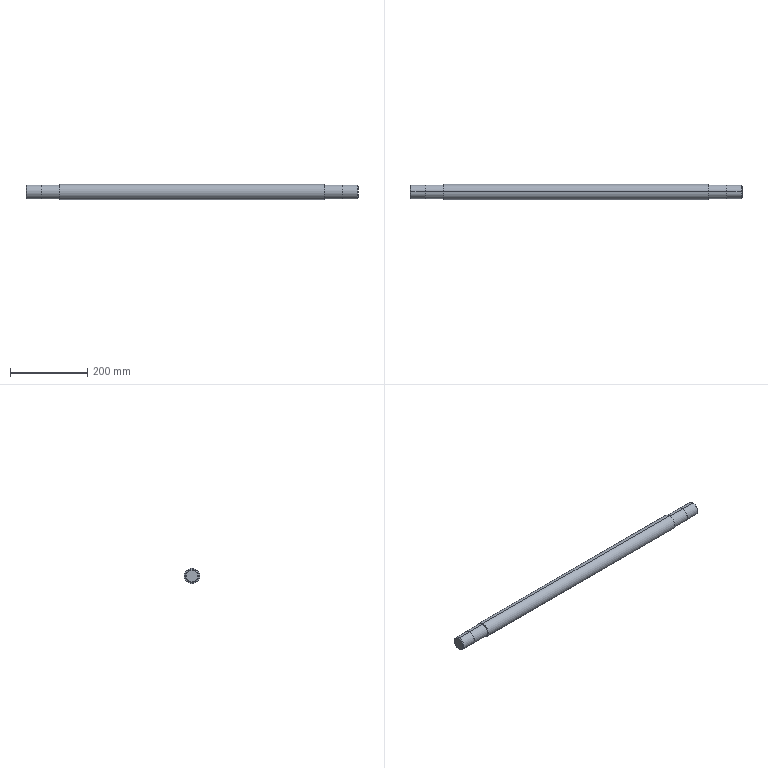Part | SolidWorks | features ICE 5, Chamfer 1, Extrusion 1 | 1 solid | 30 faces | box 861 x 40 x 40 mm | volume 1030904 mm3 | cylinder 14 | plane 12 | cone 4 | commonest cylinder face diameters 10 x4 35 x4 36 x4 40 x2
STEP:
#1=CARTESIAN_POINT('',(430.5,0.,-15.5));
#2=VERTEX_POINT('',#1);
#3=CARTESIAN_POINT('',(430.5,0.,15.5));
#4=VERTEX_POINT('',#3);
#5=CARTESIAN_POINT('',(430.5,0.,0.));
#6=DIRECTION('',(1.,0.,0.));
#7=DIRECTION('',(0.,0.,-1.));
#8=AXIS2_PLACEMENT_3D('',#5,#6,#7);
#9=CIRCLE('',#8,15.5);
#10=EDGE_CURVE('',#2,#4,#9,.T.);
#11=ORIENTED_EDGE('',*,*,#10,.F.);
#12=CARTESIAN_POINT('',(428.5,0.,-17.5));
#13=VERTEX_POINT('',#12);
#14=CARTESIAN_POINT('',(430.5,0.,-15.5));
#15=DIRECTION('',(-0.7071,0.,-0.7071));
#16=VECTOR('',#15,1000.);
#17=LINE('',#14,#16);
#18=EDGE_CURVE('',#2,#13,#17,.T.);
#19=ORIENTED_EDGE('',*,*,#18,.T.);
#20=CARTESIAN_POINT('',(428.5,0.,17.5));
#21=VERTEX_POINT('',#20);
#22=CARTESIAN_POINT('',(428.5,0.,0.));
#23=DIRECTION('',(-1.,0.,0.));
#24=DIRECTION('',(0.,0.,-1.));
#25=AXIS2_PLACEMENT_3D('',#22,#23,#24);
#26=CIRCLE('',#25,17.5);
#27=EDGE_CURVE('',#21,#13,#26,.T.);
#28=ORIENTED_EDGE('',*,*,#27,.F.);
#29=CARTESIAN_POINT('',(430.5,0.,15.5));
#30=DIRECTION('',(-0.7071,0.,0.7071));
#31=VECTOR('',#30,1000.);
#32=LINE('',#29,#31);
#33=EDGE_CURVE('',#4,#21,#32,.T.);
#34=ORIENTED_EDGE('',*,*,#33,.F.);
#35=EDGE_LOOP('',(#11,#19,#28,#34));
#36=FACE_OUTER_BOUND('',#35,.T.);
#37=CARTESIAN_POINT('',(430.5,0.,0.));
#38=DIRECTION('',(-1.,0.,0.));
#39=DIRECTION('',(0.,0.,1.));
#40=AXIS2_PLACEMENT_3D('',#37,#38,#39);
#41=CONICAL_SURFACE('',#40,15.5,0.7854);
#42=ADVANCED_FACE('',(#36),#41,.T.);
#43=CARTESIAN_POINT('',(-430.5,0.,15.5));
#44=VERTEX_POINT('',#43);
#45=CARTESIAN_POINT('',(-430.5,0.,-15.5));
#46=VERTEX_POINT('',#45);
#47=CARTESIAN_POINT('',(-430.5,0.,0.));
#48=DIRECTION('',(-1.,0.,0.));
#49=DIRECTION('',(0.,0.,1.));
#50=AXIS2_PLACEMENT_3D('',#47,#48,#49);
#51=CIRCLE('',#50,15.5);
#52=EDGE_CURVE('',#44,#46,#51,.T.);
#53=ORIENTED_EDGE('',*,*,#52,.F.);
#54=CARTESIAN_POINT('',(-428.5,0.,17.5));
#55=VERTEX_POINT('',#54);
#56=CARTESIAN_POINT('',(-430.5,0.,15.5));
#57=DIRECTION('',(0.7071,0.,0.7071));
#58=VECTOR('',#57,1000.);
#59=LINE('',#56,#58);
#60=EDGE_CURVE('',#44,#55,#59,.T.);
#61=ORIENTED_EDGE('',*,*,#60,.T.);
#62=CARTESIAN_POINT('',(-428.5,0.,-17.5));
#63=VERTEX_POINT('',#62);
#64=CARTESIAN_POINT('',(-428.5,0.,0.));
#65=DIRECTION('',(1.,0.,0.));
#66=DIRECTION('',(0.,0.,1.));
#67=AXIS2_PLACEMENT_3D('',#64,#65,#66);
#68=CIRCLE('',#67,17.5);
#69=EDGE_CURVE('',#63,#55,#68,.T.);
#70=ORIENTED_EDGE('',*,*,#69,.F.);
#71=CARTESIAN_POINT('',(-430.5,0.,-15.5));
#72=DIRECTION('',(0.7071,0.,-0.7071));
#73=VECTOR('',#72,1000.);
#74=LINE('',#71,#73);
#75=EDGE_CURVE('',#46,#63,#74,.T.);
#76=ORIENTED_EDGE('',*,*,#75,.F.);
#77=EDGE_LOOP('',(#53,#61,#70,#76));
#78=FACE_OUTER_BOUND('',#77,.T.);
#79=CARTESIAN_POINT('',(-430.5,0.,0.));
#80=DIRECTION('',(1.,0.,0.));
#81=DIRECTION('',(0.,0.,-1.));
#82=AXIS2_PLACEMENT_3D('',#79,#80,#81);
#83=CONICAL_SURFACE('',#82,15.5,0.7854);
#84=ADVANCED_FACE('',(#78),#83,.T.);
#85=ORIENTED_EDGE('',*,*,#27,.T.);
#86=CARTESIAN_POINT('',(390.5,0.,-17.5));
#87=VERTEX_POINT('',#86);
#88=CARTESIAN_POINT('',(430.5,0.,-17.5));
#89=DIRECTION('',(-1.,0.,0.));
#90=VECTOR('',#89,1000.);
#91=LINE('',#88,#90);
#92=EDGE_CURVE('',#13,#87,#91,.T.);
#93=ORIENTED_EDGE('',*,*,#92,.T.);
#94=CARTESIAN_POINT('',(390.5,0.,17.5));
#95=VERTEX_POINT('',#94);
#96=CARTESIAN_POINT('',(390.5,0.,0.));
#97=DIRECTION('',(1.,0.,0.));
#98=DIRECTION('',(0.,0.,-1.));
#99=AXIS2_PLACEMENT_3D('',#96,#97,#98);
#100=CIRCLE('',#99,17.5);
#101=EDGE_CURVE('',#87,#95,#100,.T.);
#102=ORIENTED_EDGE('',*,*,#101,.T.);
#103=CARTESIAN_POINT('',(430.5,0.,17.5));
#104=DIRECTION('',(-1.,0.,0.));
#105=VECTOR('',#104,1000.);
#106=LINE('',#103,#105);
#107=EDGE_CURVE('',#21,#95,#106,.T.);
#108=ORIENTED_EDGE('',*,*,#107,.F.);
#109=EDGE_LOOP('',(#85,#93,#102,#108));
#110=FACE_OUTER_BOUND('',#109,.T.);
#111=CARTESIAN_POINT('',(430.5,0.,0.));
#112=DIRECTION('',(-1.,0.,0.));
#113=DIRECTION('',(0.,0.,1.));
#114=AXIS2_PLACEMENT_3D('',#111,#112,#113);
#115=CYLINDRICAL_SURFACE('',#114,17.5);
#116=ADVANCED_FACE('',(#110),#115,.T.);
#117=CARTESIAN_POINT('',(351.5,17.292,-5.));
#118=VERTEX_POINT('',#117);
#119=CARTESIAN_POINT('',(381.5,17.292,-5.));
#120=VERTEX_POINT('',#119);
#121=CARTESIAN_POINT('',(390.5,17.292,-5.));
#122=DIRECTION('',(1.,0.,0.));
#123=VECTOR('',#122,1000.);
#124=LINE('',#121,#123);
#125=EDGE_CURVE('',#118,#120,#124,.T.);
#126=ORIENTED_EDGE('',*,*,#125,.T.);
#127=CARTESIAN_POINT('',(381.5,17.292,5.));
#128=VERTEX_POINT('',#127);
#129=CARTESIAN_POINT('',(381.5,17.292,-5.));
#130=CARTESIAN_POINT('',(381.827,17.292,-5.));
#131=CARTESIAN_POINT('',(382.154,17.301,-4.968));
#132=CARTESIAN_POINT('',(382.804,17.338,-4.838));
#133=CARTESIAN_POINT('',(383.116,17.364,-4.743));
#134=CARTESIAN_POINT('',(383.719,17.431,-4.493));
#135=CARTESIAN_POINT('',(384.011,17.471,-4.336));
#136=CARTESIAN_POINT('',(384.553,17.557,-3.973));
#137=CARTESIAN_POINT('',(384.804,17.603,-3.767));
#138=CARTESIAN_POINT('',(385.265,17.695,-3.306));
#139=CARTESIAN_POINT('',(385.474,17.742,-3.051));
#140=CARTESIAN_POINT('',(385.835,17.826,-2.512));
#141=CARTESIAN_POINT('',(385.99,17.865,-2.225));
#142=CARTESIAN_POINT('',(386.243,17.93,-1.616));
#143=CARTESIAN_POINT('',(386.338,17.956,-1.302));
#144=CARTESIAN_POINT('',(386.435,17.982,-0.8219));
#145=CARTESIAN_POINT('',(386.459,17.989,-0.66));
#146=CARTESIAN_POINT('',(386.492,17.998,-0.3322));
#147=CARTESIAN_POINT('',(386.5,18.,-0.1657));
#148=CARTESIAN_POINT('',(386.5,18.,0.3288));
#149=CARTESIAN_POINT('',(386.468,17.991,0.6544));
#150=CARTESIAN_POINT('',(386.34,17.956,1.298));
#151=CARTESIAN_POINT('',(386.243,17.93,1.617));
#152=CARTESIAN_POINT('',(385.992,17.865,2.219));
#153=CARTESIAN_POINT('',(385.839,17.827,2.507));
#154=CARTESIAN_POINT('',(385.474,17.741,3.053));
#155=CARTESIAN_POINT('',(385.266,17.696,3.305));
#156=CARTESIAN_POINT('',(384.922,17.627,3.649));
#157=CARTESIAN_POINT('',(384.802,17.604,3.758));
#158=CARTESIAN_POINT('',(384.55,17.558,3.965));
#159=CARTESIAN_POINT('',(384.417,17.535,4.064));
#160=CARTESIAN_POINT('',(384.01,17.471,4.337));
#161=CARTESIAN_POINT('',(383.724,17.431,4.49));
#162=CARTESIAN_POINT('',(383.122,17.365,4.741));
#163=CARTESIAN_POINT('',(382.803,17.338,4.838));
#164=CARTESIAN_POINT('',(382.159,17.301,4.967));
#165=CARTESIAN_POINT('',(381.832,17.292,5.));
#166=CARTESIAN_POINT('',(381.5,17.292,5.));
#167=B_SPLINE_CURVE_WITH_KNOTS('',3,(#129,#130,#131,#132,#133,#134,#135,#136,#137,#138,#139,#140,#141,#142,#143,#144,#145,#146,#147,#148,#149,#150,#151,#152,#153,#154,#155,#156,#157,#158,#159,#160,#161,#162,#163,#164,#165,#166),.UNSPECIFIED.,.F.,.F.,(4,2,2,2,2,2,2,2,2,2,2,2,2,2,2,2,2,2,4),(0.01571,0.01669,0.01767,0.01865,0.01964,0.02062,0.0216,0.02258,0.02307,0.02356,0.02454,0.02553,0.02651,0.02749,0.02798,0.02847,0.02945,0.03043,0.03142),.UNSPECIFIED.);
#168=EDGE_CURVE('',#120,#128,#167,.T.);
#169=ORIENTED_EDGE('',*,*,#168,.T.);
#170=CARTESIAN_POINT('',(351.5,17.292,5.));
#171=VERTEX_POINT('',#170);
#172=CARTESIAN_POINT('',(390.5,17.292,5.));
#173=DIRECTION('',(-1.,0.,0.));
#174=VECTOR('',#173,1000.);
#175=LINE('',#172,#174);
#176=EDGE_CURVE('',#128,#171,#175,.T.);
#177=ORIENTED_EDGE('',*,*,#176,.T.);
#178=CARTESIAN_POINT('',(351.5,17.292,5.));
#179=CARTESIAN_POINT('',(351.168,17.292,5.));
#180=CARTESIAN_POINT('',(350.842,17.301,4.967));
#181=CARTESIAN_POINT('',(350.201,17.337,4.839));
#182=CARTESIAN_POINT('',(349.882,17.365,4.742));
#183=CARTESIAN_POINT('',(349.278,17.431,4.491));
#184=CARTESIAN_POINT('',(348.991,17.471,4.337));
#185=CARTESIAN_POINT('',(348.449,17.557,3.975));
#186=CARTESIAN_POINT('',(348.194,17.603,3.765));
#187=CARTESIAN_POINT('',(347.735,17.695,3.306));
#188=CARTESIAN_POINT('',(347.529,17.741,3.056));
#189=CARTESIAN_POINT('',(347.163,17.826,2.51));
#190=CARTESIAN_POINT('',(347.009,17.865,2.222));
#191=CARTESIAN_POINT('',(346.821,17.913,1.771));
#192=CARTESIAN_POINT('',(346.766,17.928,1.618));
#193=CARTESIAN_POINT('',(346.67,17.953,1.304));
#194=CARTESIAN_POINT('',(346.63,17.964,1.143));
#195=CARTESIAN_POINT('',(346.533,17.991,0.658));
#196=CARTESIAN_POINT('',(346.5,18.,0.3326));
#197=CARTESIAN_POINT('',(346.5,18.,-0.3232));
#198=CARTESIAN_POINT('',(346.532,17.991,-0.6563));
#199=CARTESIAN_POINT('',(346.661,17.956,-1.299));
#200=CARTESIAN_POINT('',(346.755,17.93,-1.611));
#201=CARTESIAN_POINT('',(347.007,17.865,-2.219));
#202=CARTESIAN_POINT('',(347.163,17.826,-2.509));
#203=CARTESIAN_POINT('',(347.524,17.742,-3.049));
#204=CARTESIAN_POINT('',(347.732,17.696,-3.303));
#205=CARTESIAN_POINT('',(348.194,17.603,-3.765));
#206=CARTESIAN_POINT('',(348.445,17.557,-3.971));
#207=CARTESIAN_POINT('',(348.985,17.472,-4.333));
#208=CARTESIAN_POINT('',(349.277,17.431,-4.491));
#209=CARTESIAN_POINT('',(349.88,17.365,-4.741));
#210=CARTESIAN_POINT('',(350.191,17.338,-4.837));
#211=CARTESIAN_POINT('',(350.836,17.301,-4.967));
#212=CARTESIAN_POINT('',(351.168,17.292,-5.));
#213=CARTESIAN_POINT('',(351.5,17.292,-5.));
#214=B_SPLINE_CURVE_WITH_KNOTS('',3,(#178,#179,#180,#181,#182,#183,#184,#185,#186,#187,#188,#189,#190,#191,#192,#193,#194,#195,#196,#197,#198,#199,#200,#201,#202,#203,#204,#205,#206,#207,#208,#209,#210,#211,#212,#213),.UNSPECIFIED.,.F.,.F.,(4,2,2,2,2,2,2,2,2,2,2,2,2,2,2,2,2,4),(0.,0.0009815,0.001963,0.002945,0.003926,0.004908,0.005889,0.00638,0.006871,0.007852,0.008834,0.009815,0.0108,0.01178,0.01276,0.01374,0.01472,0.0157),.UNSPECIFIED.);
#215=EDGE_CURVE('',#171,#118,#214,.T.);
#216=ORIENTED_EDGE('',*,*,#215,.T.);
#217=EDGE_LOOP('',(#126,#169,#177,#216));
#218=FACE_BOUND('',#217,.T.);
#219=CARTESIAN_POINT('',(390.5,0.,-18.));
#220=VERTEX_POINT('',#219);
#221=CARTESIAN_POINT('',(390.5,0.,18.));
#222=VERTEX_POINT('',#221);
#223=CARTESIAN_POINT('',(390.5,0.,0.));
#224=DIRECTION('',(1.,0.,0.));
#225=DIRECTION('',(0.,0.,-1.));
#226=AXIS2_PLACEMENT_3D('',#223,#224,#225);
#227=CIRCLE('',#226,18.);
#228=EDGE_CURVE('',#220,#222,#227,.T.);
#229=ORIENTED_EDGE('',*,*,#228,.F.);
#230=CARTESIAN_POINT('',(342.5,0.,-18.));
#231=VERTEX_POINT('',#230);
#232=CARTESIAN_POINT('',(390.5,0.,-18.));
#233=DIRECTION('',(-1.,0.,0.));
#234=VECTOR('',#233,1000.);
#235=LINE('',#232,#234);
#236=EDGE_CURVE('',#220,#231,#235,.T.);
#237=ORIENTED_EDGE('',*,*,#236,.T.);
#238=CARTESIAN_POINT('',(342.5,0.,18.));
#239=VERTEX_POINT('',#238);
#240=CARTESIAN_POINT('',(342.5,0.,0.));
#241=DIRECTION('',(1.,0.,0.));
#242=DIRECTION('',(0.,0.,-1.));
#243=AXIS2_PLACEMENT_3D('',#240,#241,#242);
#244=CIRCLE('',#243,18.);
#245=EDGE_CURVE('',#231,#239,#244,.T.);
#246=ORIENTED_EDGE('',*,*,#245,.T.);
#247=CARTESIAN_POINT('',(390.5,0.,18.));
#248=DIRECTION('',(-1.,0.,0.));
#249=VECTOR('',#248,1000.);
#250=LINE('',#247,#249);
#251=EDGE_CURVE('',#222,#239,#250,.T.);
#252=ORIENTED_EDGE('',*,*,#251,.F.);
#253=EDGE_LOOP('',(#229,#237,#246,#252));
#254=FACE_OUTER_BOUND('',#253,.T.);
#255=CARTESIAN_POINT('',(390.5,0.,0.));
#256=DIRECTION('',(-1.,0.,0.));
#257=DIRECTION('',(0.,0.,1.));
#258=AXIS2_PLACEMENT_3D('',#255,#256,#257);
#259=CYLINDRICAL_SURFACE('',#258,18.);
#260=ADVANCED_FACE('',(#218,#254),#259,.T.);
#261=ORIENTED_EDGE('',*,*,#69,.T.);
#262=CARTESIAN_POINT('',(-390.5,0.,17.5));
#263=VERTEX_POINT('',#262);
#264=CARTESIAN_POINT('',(-430.5,0.,17.5));
#265=DIRECTION('',(1.,0.,0.));
#266=VECTOR('',#265,1000.);
#267=LINE('',#264,#266);
#268=EDGE_CURVE('',#55,#263,#267,.T.);
#269=ORIENTED_EDGE('',*,*,#268,.T.);
#270=CARTESIAN_POINT('',(-390.5,0.,-17.5));
#271=VERTEX_POINT('',#270);
#272=CARTESIAN_POINT('',(-390.5,0.,0.));
#273=DIRECTION('',(-1.,0.,0.));
#274=DIRECTION('',(0.,0.,1.));
#275=AXIS2_PLACEMENT_3D('',#272,#273,#274);
#276=CIRCLE('',#275,17.5);
#277=EDGE_CURVE('',#263,#271,#276,.T.);
#278=ORIENTED_EDGE('',*,*,#277,.T.);
#279=CARTESIAN_POINT('',(-430.5,0.,-17.5));
#280=DIRECTION('',(1.,0.,0.));
#281=VECTOR('',#280,1000.);
#282=LINE('',#279,#281);
#283=EDGE_CURVE('',#63,#271,#282,.T.);
#284=ORIENTED_EDGE('',*,*,#283,.F.);
#285=EDGE_LOOP('',(#261,#269,#278,#284));
#286=FACE_OUTER_BOUND('',#285,.T.);
#287=CARTESIAN_POINT('',(-430.5,0.,0.));
#288=DIRECTION('',(1.,0.,0.));
#289=DIRECTION('',(0.,0.,-1.));
#290=AXIS2_PLACEMENT_3D('',#287,#288,#289);
#291=CYLINDRICAL_SURFACE('',#290,17.5);
#292=ADVANCED_FACE('',(#286),#291,.T.);
#293=CARTESIAN_POINT('',(-351.5,17.292,5.));
#294=VERTEX_POINT('',#293);
#295=CARTESIAN_POINT('',(-381.5,17.292,5.));
#296=VERTEX_POINT('',#295);
#297=CARTESIAN_POINT('',(-390.5,17.292,5.));
#298=DIRECTION('',(-1.,0.,0.));
#299=VECTOR('',#298,1000.);
#300=LINE('',#297,#299);
#301=EDGE_CURVE('',#294,#296,#300,.T.);
#302=ORIENTED_EDGE('',*,*,#301,.T.);
#303=CARTESIAN_POINT('',(-381.5,17.292,-5.));
#304=VERTEX_POINT('',#303);
#305=CARTESIAN_POINT('',(-381.5,17.292,5.));
#306=CARTESIAN_POINT('',(-381.832,17.292,5.));
#307=CARTESIAN_POINT('',(-382.158,17.301,4.967));
#308=CARTESIAN_POINT('',(-382.799,17.337,4.839));
#309=CARTESIAN_POINT('',(-383.118,17.365,4.742));
#310=CARTESIAN_POINT('',(-383.722,17.431,4.491));
#311=CARTESIAN_POINT('',(-384.009,17.471,4.337));
#312=CARTESIAN_POINT('',(-384.551,17.557,3.975));
#313=CARTESIAN_POINT('',(-384.806,17.603,3.765));
#314=CARTESIAN_POINT('',(-385.265,17.695,3.306));
#315=CARTESIAN_POINT('',(-385.471,17.741,3.056));
#316=CARTESIAN_POINT('',(-385.837,17.826,2.51));
#317=CARTESIAN_POINT('',(-385.991,17.865,2.222));
#318=CARTESIAN_POINT('',(-386.179,17.913,1.771));
#319=CARTESIAN_POINT('',(-386.234,17.928,1.618));
#320=CARTESIAN_POINT('',(-386.33,17.953,1.304));
#321=CARTESIAN_POINT('',(-386.37,17.964,1.143));
#322=CARTESIAN_POINT('',(-386.467,17.991,0.658));
#323=CARTESIAN_POINT('',(-386.5,18.,0.3326));
#324=CARTESIAN_POINT('',(-386.5,18.,-0.3232));
#325=CARTESIAN_POINT('',(-386.468,17.991,-0.6563));
#326=CARTESIAN_POINT('',(-386.339,17.956,-1.299));
#327=CARTESIAN_POINT('',(-386.245,17.93,-1.611));
#328=CARTESIAN_POINT('',(-385.993,17.865,-2.219));
#329=CARTESIAN_POINT('',(-385.837,17.826,-2.509));
#330=CARTESIAN_POINT('',(-385.476,17.742,-3.049));
#331=CARTESIAN_POINT('',(-385.268,17.696,-3.303));
#332=CARTESIAN_POINT('',(-384.806,17.603,-3.765));
#333=CARTESIAN_POINT('',(-384.555,17.557,-3.971));
#334=CARTESIAN_POINT('',(-384.015,17.472,-4.333));
#335=CARTESIAN_POINT('',(-383.723,17.431,-4.491));
#336=CARTESIAN_POINT('',(-383.12,17.365,-4.741));
#337=CARTESIAN_POINT('',(-382.809,17.338,-4.837));
#338=CARTESIAN_POINT('',(-382.164,17.301,-4.967));
#339=CARTESIAN_POINT('',(-381.832,17.292,-5.));
#340=CARTESIAN_POINT('',(-381.5,17.292,-5.));
#341=B_SPLINE_CURVE_WITH_KNOTS('',3,(#305,#306,#307,#308,#309,#310,#311,#312,#313,#314,#315,#316,#317,#318,#319,#320,#321,#322,#323,#324,#325,#326,#327,#328,#329,#330,#331,#332,#333,#334,#335,#336,#337,#338,#339,#340),.UNSPECIFIED.,.F.,.F.,(4,2,2,2,2,2,2,2,2,2,2,2,2,2,2,2,2,4),(0.,0.0009815,0.001963,0.002945,0.003926,0.004908,0.005889,0.00638,0.006871,0.007852,0.008834,0.009815,0.0108,0.01178,0.01276,0.01374,0.01472,0.0157),.UNSPECIFIED.);
#342=EDGE_CURVE('',#296,#304,#341,.T.);
#343=ORIENTED_EDGE('',*,*,#342,.T.);
#344=CARTESIAN_POINT('',(-351.5,17.292,-5.));
#345=VERTEX_POINT('',#344);
#346=CARTESIAN_POINT('',(-390.5,17.292,-5.));
#347=DIRECTION('',(1.,0.,0.));
#348=VECTOR('',#347,1000.);
#349=LINE('',#346,#348);
#350=EDGE_CURVE('',#304,#345,#349,.T.);
#351=ORIENTED_EDGE('',*,*,#350,.T.);
#352=CARTESIAN_POINT('',(-351.5,17.292,-5.));
#353=CARTESIAN_POINT('',(-351.173,17.292,-5.));
#354=CARTESIAN_POINT('',(-350.846,17.301,-4.968));
#355=CARTESIAN_POINT('',(-350.196,17.338,-4.838));
#356=CARTESIAN_POINT('',(-349.884,17.364,-4.743));
#357=CARTESIAN_POINT('',(-349.281,17.431,-4.493));
#358=CARTESIAN_POINT('',(-348.989,17.471,-4.336));
#359=CARTESIAN_POINT('',(-348.447,17.557,-3.973));
#360=CARTESIAN_POINT('',(-348.196,17.603,-3.767));
#361=CARTESIAN_POINT('',(-347.735,17.695,-3.306));
#362=CARTESIAN_POINT('',(-347.526,17.742,-3.051));
#363=CARTESIAN_POINT('',(-347.165,17.826,-2.512));
#364=CARTESIAN_POINT('',(-347.01,17.865,-2.225));
#365=CARTESIAN_POINT('',(-346.757,17.93,-1.616));
#366=CARTESIAN_POINT('',(-346.662,17.956,-1.302));
#367=CARTESIAN_POINT('',(-346.565,17.982,-0.8219));
#368=CARTESIAN_POINT('',(-346.541,17.989,-0.66));
#369=CARTESIAN_POINT('',(-346.508,17.998,-0.3322));
#370=CARTESIAN_POINT('',(-346.5,18.,-0.1657));
#371=CARTESIAN_POINT('',(-346.5,18.,0.3288));
#372=CARTESIAN_POINT('',(-346.532,17.991,0.6544));
#373=CARTESIAN_POINT('',(-346.66,17.956,1.298));
#374=CARTESIAN_POINT('',(-346.757,17.93,1.617));
#375=CARTESIAN_POINT('',(-347.008,17.865,2.219));
#376=CARTESIAN_POINT('',(-347.161,17.827,2.507));
#377=CARTESIAN_POINT('',(-347.526,17.741,3.053));
#378=CARTESIAN_POINT('',(-347.734,17.696,3.305));
#379=CARTESIAN_POINT('',(-348.078,17.627,3.649));
#380=CARTESIAN_POINT('',(-348.198,17.604,3.758));
#381=CARTESIAN_POINT('',(-348.45,17.558,3.965));
#382=CARTESIAN_POINT('',(-348.583,17.535,4.064));
#383=CARTESIAN_POINT('',(-348.99,17.471,4.337));
#384=CARTESIAN_POINT('',(-349.276,17.431,4.49));
#385=CARTESIAN_POINT('',(-349.878,17.365,4.741));
#386=CARTESIAN_POINT('',(-350.197,17.338,4.838));
#387=CARTESIAN_POINT('',(-350.841,17.301,4.967));
#388=CARTESIAN_POINT('',(-351.168,17.292,5.));
#389=CARTESIAN_POINT('',(-351.5,17.292,5.));
#390=B_SPLINE_CURVE_WITH_KNOTS('',3,(#352,#353,#354,#355,#356,#357,#358,#359,#360,#361,#362,#363,#364,#365,#366,#367,#368,#369,#370,#371,#372,#373,#374,#375,#376,#377,#378,#379,#380,#381,#382,#383,#384,#385,#386,#387,#388,#389),.UNSPECIFIED.,.F.,.F.,(4,2,2,2,2,2,2,2,2,2,2,2,2,2,2,2,2,2,4),(0.01571,0.01669,0.01767,0.01865,0.01964,0.02062,0.0216,0.02258,0.02307,0.02356,0.02454,0.02553,0.02651,0.02749,0.02798,0.02847,0.02945,0.03043,0.03142),.UNSPECIFIED.);
#391=EDGE_CURVE('',#345,#294,#390,.T.);
#392=ORIENTED_EDGE('',*,*,#391,.T.);
#393=EDGE_LOOP('',(#302,#343,#351,#392));
#394=FACE_BOUND('',#393,.T.);
#395=CARTESIAN_POINT('',(-390.5,0.,18.));
#396=VERTEX_POINT('',#395);
#397=CARTESIAN_POINT('',(-390.5,0.,-18.));
#398=VERTEX_POINT('',#397);
#399=CARTESIAN_POINT('',(-390.5,0.,0.));
#400=DIRECTION('',(-1.,0.,0.));
#401=DIRECTION('',(0.,0.,1.));
#402=AXIS2_PLACEMENT_3D('',#399,#400,#401);
#403=CIRCLE('',#402,18.);
#404=EDGE_CURVE('',#396,#398,#403,.T.);
#405=ORIENTED_EDGE('',*,*,#404,.F.);
#406=CARTESIAN_POINT('',(-342.5,0.,18.));
#407=VERTEX_POINT('',#406);
#408=CARTESIAN_POINT('',(-390.5,0.,18.));
#409=DIRECTION('',(1.,0.,0.));
#410=VECTOR('',#409,1000.);
#411=LINE('',#408,#410);
#412=EDGE_CURVE('',#396,#407,#411,.T.);
#413=ORIENTED_EDGE('',*,*,#412,.T.);
#414=CARTESIAN_POINT('',(-342.5,0.,-18.));
#415=VERTEX_POINT('',#414);
#416=CARTESIAN_POINT('',(-342.5,0.,0.));
#417=DIRECTION('',(-1.,0.,0.));
#418=DIRECTION('',(0.,0.,-1.));
#419=AXIS2_PLACEMENT_3D('',#416,#417,#418);
#420=CIRCLE('',#419,18.);
#421=EDGE_CURVE('',#407,#415,#420,.T.);
#422=ORIENTED_EDGE('',*,*,#421,.T.);
#423=CARTESIAN_POINT('',(-390.5,0.,-18.));
#424=DIRECTION('',(1.,0.,0.));
#425=VECTOR('',#424,1000.);
#426=LINE('',#423,#425);
#427=EDGE_CURVE('',#398,#415,#426,.T.);
#428=ORIENTED_EDGE('',*,*,#427,.F.);
#429=EDGE_LOOP('',(#405,#413,#422,#428));
#430=FACE_OUTER_BOUND('',#429,.T.);
#431=CARTESIAN_POINT('',(-390.5,0.,0.));
#432=DIRECTION('',(1.,0.,0.));
#433=DIRECTION('',(0.,0.,-1.));
#434=AXIS2_PLACEMENT_3D('',#431,#432,#433);
#435=CYLINDRICAL_SURFACE('',#434,18.);
#436=ADVANCED_FACE('',(#394,#430),#435,.T.);
#437=CARTESIAN_POINT('',(342.5,0.,-20.));
#438=VERTEX_POINT('',#437);
#439=CARTESIAN_POINT('',(342.5,0.,20.));
#440=VERTEX_POINT('',#439);
#441=CARTESIAN_POINT('',(342.5,0.,0.));
#442=DIRECTION('',(1.,0.,0.));
#443=DIRECTION('',(0.,0.,-1.));
#444=AXIS2_PLACEMENT_3D('',#441,#442,#443);
#445=CIRCLE('',#444,20.);
#446=EDGE_CURVE('',#438,#440,#445,.T.);
#447=ORIENTED_EDGE('',*,*,#446,.F.);
#448=CARTESIAN_POINT('',(-342.5,0.,-20.));
#449=VERTEX_POINT('',#448);
#450=CARTESIAN_POINT('',(342.5,0.,-20.));
#451=DIRECTION('',(-1.,0.,0.));
#452=VECTOR('',#451,1000.);
#453=LINE('',#450,#452);
#454=EDGE_CURVE('',#438,#449,#453,.T.);
#455=ORIENTED_EDGE('',*,*,#454,.T.);
#456=CARTESIAN_POINT('',(-342.5,0.,20.));
#457=VERTEX_POINT('',#456);
#458=CARTESIAN_POINT('',(-342.5,0.,0.));
#459=DIRECTION('',(1.,0.,0.));
#460=DIRECTION('',(0.,0.,-1.));
#461=AXIS2_PLACEMENT_3D('',#458,#459,#460);
#462=CIRCLE('',#461,20.);
#463=EDGE_CURVE('',#449,#457,#462,.T.);
#464=ORIENTED_EDGE('',*,*,#463,.T.);
#465=CARTESIAN_POINT('',(342.5,0.,20.));
#466=DIRECTION('',(-1.,0.,0.));
#467=VECTOR('',#466,1000.);
#468=LINE('',#465,#467);
#469=EDGE_CURVE('',#440,#457,#468,.T.);
#470=ORIENTED_EDGE('',*,*,#469,.F.);
#471=EDGE_LOOP('',(#447,#455,#464,#470));
#472=FACE_OUTER_BOUND('',#471,.T.);
#473=CARTESIAN_POINT('',(342.5,0.,0.));
#474=DIRECTION('',(-1.,0.,0.));
#475=DIRECTION('',(0.,0.,1.));
#476=AXIS2_PLACEMENT_3D('',#473,#474,#475);
#477=CYLINDRICAL_SURFACE('',#476,20.);
#478=ADVANCED_FACE('',(#472),#477,.T.);
#479=CARTESIAN_POINT('',(390.5,0.,0.));
#480=DIRECTION('',(1.,0.,0.));
#481=DIRECTION('',(0.,0.,-1.));
#482=AXIS2_PLACEMENT_3D('',#479,#480,#481);
#483=CIRCLE('',#482,18.);
#484=EDGE_CURVE('',#222,#220,#483,.T.);
#485=ORIENTED_EDGE('',*,*,#484,.T.);
#486=ORIENTED_EDGE('',*,*,#228,.T.);
#487=EDGE_LOOP('',(#485,#486));
#488=FACE_OUTER_BOUND('',#487,.T.);
#489=CARTESIAN_POINT('',(390.5,0.,0.));
#490=DIRECTION('',(1.,0.,0.));
#491=DIRECTION('',(0.,0.,-1.));
#492=AXIS2_PLACEMENT_3D('',#489,#490,#491);
#493=CIRCLE('',#492,17.5);
#494=EDGE_CURVE('',#95,#87,#493,.T.);
#495=ORIENTED_EDGE('',*,*,#494,.F.);
#496=ORIENTED_EDGE('',*,*,#101,.F.);
#497=EDGE_LOOP('',(#495,#496));
#498=FACE_BOUND('',#497,.T.);
#499=CARTESIAN_POINT('',(390.5,0.,0.));
#500=DIRECTION('',(1.,0.,0.));
#501=DIRECTION('',(0.,0.,-1.));
#502=AXIS2_PLACEMENT_3D('',#499,#500,#501);
#503=PLANE('',#502);
#504=ADVANCED_FACE('',(#488,#498),#503,.T.);
#505=CARTESIAN_POINT('',(342.5,0.,0.));
#506=DIRECTION('',(1.,0.,0.));
#507=DIRECTION('',(0.,0.,-1.));
#508=AXIS2_PLACEMENT_3D('',#505,#506,#507);
#509=CIRCLE('',#508,20.);
#510=EDGE_CURVE('',#440,#438,#509,.T.);
#511=ORIENTED_EDGE('',*,*,#510,.T.);
#512=ORIENTED_EDGE('',*,*,#446,.T.);
#513=EDGE_LOOP('',(#511,#512));
#514=FACE_OUTER_BOUND('',#513,.T.);
#515=CARTESIAN_POINT('',(342.5,0.,0.));
#516=DIRECTION('',(1.,0.,0.));
#517=DIRECTION('',(0.,0.,-1.));
#518=AXIS2_PLACEMENT_3D('',#515,#516,#517);
#519=CIRCLE('',#518,18.);
#520=EDGE_CURVE('',#239,#231,#519,.T.);
#521=ORIENTED_EDGE('',*,*,#520,.F.);
#522=ORIENTED_EDGE('',*,*,#245,.F.);
#523=EDGE_LOOP('',(#521,#522));
#524=FACE_BOUND('',#523,.T.);
#525=CARTESIAN_POINT('',(342.5,0.,0.));
#526=DIRECTION('',(1.,0.,0.));
#527=DIRECTION('',(0.,0.,-1.));
#528=AXIS2_PLACEMENT_3D('',#525,#526,#527);
#529=PLANE('',#528);
#530=ADVANCED_FACE('',(#514,#524),#529,.T.);
#531=CARTESIAN_POINT('',(-390.5,0.,0.));
#532=DIRECTION('',(-1.,0.,0.));
#533=DIRECTION('',(0.,0.,1.));
#534=AXIS2_PLACEMENT_3D('',#531,#532,#533);
#535=CIRCLE('',#534,18.);
#536=EDGE_CURVE('',#398,#396,#535,.T.);
#537=ORIENTED_EDGE('',*,*,#536,.T.);
#538=ORIENTED_EDGE('',*,*,#404,.T.);
#539=EDGE_LOOP('',(#537,#538));
#540=FACE_OUTER_BOUND('',#539,.T.);
#541=CARTESIAN_POINT('',(-390.5,0.,0.));
#542=DIRECTION('',(-1.,0.,0.));
#543=DIRECTION('',(0.,0.,1.));
#544=AXIS2_PLACEMENT_3D('',#541,#542,#543);
#545=CIRCLE('',#544,17.5);
#546=EDGE_CURVE('',#271,#263,#545,.T.);
#547=ORIENTED_EDGE('',*,*,#546,.F.);
#548=ORIENTED_EDGE('',*,*,#277,.F.);
#549=EDGE_LOOP('',(#547,#548));
#550=FACE_BOUND('',#549,.T.);
#551=CARTESIAN_POINT('',(-390.5,0.,0.));
#552=DIRECTION('',(-1.,0.,0.));
#553=DIRECTION('',(0.,0.,1.));
#554=AXIS2_PLACEMENT_3D('',#551,#552,#553);
#555=PLANE('',#554);
#556=ADVANCED_FACE('',(#540,#550),#555,.T.);
#557=CARTESIAN_POINT('',(-342.5,0.,0.));
#558=DIRECTION('',(1.,0.,0.));
#559=DIRECTION('',(0.,0.,-1.));
#560=AXIS2_PLACEMENT_3D('',#557,#558,#559);
#561=CIRCLE('',#560,20.);
#562=EDGE_CURVE('',#457,#449,#561,.T.);
#563=ORIENTED_EDGE('',*,*,#562,.F.);
#564=ORIENTED_EDGE('',*,*,#463,.F.);
#565=EDGE_LOOP('',(#563,#564));
#566=FACE_OUTER_BOUND('',#565,.T.);
#567=CARTESIAN_POINT('',(-342.5,0.,0.));
#568=DIRECTION('',(-1.,0.,0.));
#569=DIRECTION('',(0.,0.,-1.));
#570=AXIS2_PLACEMENT_3D('',#567,#568,#569);
#571=CIRCLE('',#570,18.);
#572=EDGE_CURVE('',#415,#407,#571,.T.);
#573=ORIENTED_EDGE('',*,*,#572,.F.);
#574=ORIENTED_EDGE('',*,*,#421,.F.);
#575=EDGE_LOOP('',(#573,#574));
#576=FACE_BOUND('',#575,.T.);
#577=CARTESIAN_POINT('',(-342.5,0.,0.));
#578=DIRECTION('',(1.,0.,0.));
#579=DIRECTION('',(0.,0.,-1.));
#580=AXIS2_PLACEMENT_3D('',#577,#578,#579);
#581=PLANE('',#580);
#582=ADVANCED_FACE('',(#566,#576),#581,.F.);
#583=ORIENTED_EDGE('',*,*,#454,.F.);
#584=ORIENTED_EDGE('',*,*,#510,.F.);
#585=ORIENTED_EDGE('',*,*,#469,.T.);
#586=ORIENTED_EDGE('',*,*,#562,.T.);
#587=EDGE_LOOP('',(#583,#584,#585,#586));
#588=FACE_OUTER_BOUND('',#587,.T.);
#589=CARTESIAN_POINT('',(342.5,0.,0.));
#590=DIRECTION('',(-1.,0.,0.));
#591=DIRECTION('',(0.,0.,1.));
#592=AXIS2_PLACEMENT_3D('',#589,#590,#591);
#593=CYLINDRICAL_SURFACE('',#592,20.);
#594=ADVANCED_FACE('',(#588),#593,.T.);
#595=ORIENTED_EDGE('',*,*,#412,.F.);
#596=ORIENTED_EDGE('',*,*,#536,.F.);
#597=ORIENTED_EDGE('',*,*,#427,.T.);
#598=ORIENTED_EDGE('',*,*,#572,.T.);
#599=EDGE_LOOP('',(#595,#596,#597,#598));
#600=FACE_OUTER_BOUND('',#599,.T.);
#601=CARTESIAN_POINT('',(-390.5,0.,0.));
#602=DIRECTION('',(1.,0.,0.));
#603=DIRECTION('',(0.,0.,-1.));
#604=AXIS2_PLACEMENT_3D('',#601,#602,#603);
#605=CYLINDRICAL_SURFACE('',#604,18.);
#606=ADVANCED_FACE('',(#600),#605,.T.);
#607=ORIENTED_EDGE('',*,*,#268,.F.);
#608=CARTESIAN_POINT('',(-428.5,0.,0.));
#609=DIRECTION('',(1.,0.,0.));
#610=DIRECTION('',(0.,0.,1.));
#611=AXIS2_PLACEMENT_3D('',#608,#609,#610);
#612=CIRCLE('',#611,17.5);
#613=EDGE_CURVE('',#55,#63,#612,.T.);
#614=ORIENTED_EDGE('',*,*,#613,.T.);
#615=ORIENTED_EDGE('',*,*,#283,.T.);
#616=ORIENTED_EDGE('',*,*,#546,.T.);
#617=EDGE_LOOP('',(#607,#614,#615,#616));
#618=FACE_OUTER_BOUND('',#617,.T.);
#619=CARTESIAN_POINT('',(-430.5,0.,0.));
#620=DIRECTION('',(1.,0.,0.));
#621=DIRECTION('',(0.,0.,-1.));
#622=AXIS2_PLACEMENT_3D('',#619,#620,#621);
#623=CYLINDRICAL_SURFACE('',#622,17.5);
#624=ADVANCED_FACE('',(#618),#623,.T.);
#625=CARTESIAN_POINT('',(-430.5,0.,0.));
#626=DIRECTION('',(-1.,0.,0.));
#627=DIRECTION('',(0.,0.,1.));
#628=AXIS2_PLACEMENT_3D('',#625,#626,#627);
#629=CIRCLE('',#628,15.5);
#630=EDGE_CURVE('',#46,#44,#629,.T.);
#631=ORIENTED_EDGE('',*,*,#630,.T.);
#632=ORIENTED_EDGE('',*,*,#52,.T.);
#633=EDGE_LOOP('',(#631,#632));
#634=FACE_OUTER_BOUND('',#633,.T.);
#635=CARTESIAN_POINT('',(-430.5,0.,0.));
#636=DIRECTION('',(-1.,0.,0.));
#637=DIRECTION('',(0.,0.,1.));
#638=AXIS2_PLACEMENT_3D('',#635,#636,#637);
#639=PLANE('',#638);
#640=ADVANCED_FACE('',(#634),#639,.T.);
#641=ORIENTED_EDGE('',*,*,#236,.F.);
#642=ORIENTED_EDGE('',*,*,#484,.F.);
#643=ORIENTED_EDGE('',*,*,#251,.T.);
#644=ORIENTED_EDGE('',*,*,#520,.T.);
#645=EDGE_LOOP('',(#641,#642,#643,#644));
#646=FACE_OUTER_BOUND('',#645,.T.);
#647=CARTESIAN_POINT('',(390.5,0.,0.));
#648=DIRECTION('',(-1.,0.,0.));
#649=DIRECTION('',(0.,0.,1.));
#650=AXIS2_PLACEMENT_3D('',#647,#648,#649);
#651=CYLINDRICAL_SURFACE('',#650,18.);
#652=ADVANCED_FACE('',(#646),#651,.T.);
#653=ORIENTED_EDGE('',*,*,#92,.F.);
#654=CARTESIAN_POINT('',(428.5,0.,0.));
#655=DIRECTION('',(-1.,0.,0.));
#656=DIRECTION('',(0.,0.,-1.));
#657=AXIS2_PLACEMENT_3D('',#654,#655,#656);
#658=CIRCLE('',#657,17.5);
#659=EDGE_CURVE('',#13,#21,#658,.T.);
#660=ORIENTED_EDGE('',*,*,#659,.T.);
#661=ORIENTED_EDGE('',*,*,#107,.T.);
#662=ORIENTED_EDGE('',*,*,#494,.T.);
#663=EDGE_LOOP('',(#653,#660,#661,#662));
#664=FACE_OUTER_BOUND('',#663,.T.);
#665=CARTESIAN_POINT('',(430.5,0.,0.));
#666=DIRECTION('',(-1.,0.,0.));
#667=DIRECTION('',(0.,0.,1.));
#668=AXIS2_PLACEMENT_3D('',#665,#666,#667);
#669=CYLINDRICAL_SURFACE('',#668,17.5);
#670=ADVANCED_FACE('',(#664),#669,.T.);
#671=CARTESIAN_POINT('',(430.5,0.,0.));
#672=DIRECTION('',(1.,0.,0.));
#673=DIRECTION('',(0.,0.,-1.));
#674=AXIS2_PLACEMENT_3D('',#671,#672,#673);
#675=CIRCLE('',#674,15.5);
#676=EDGE_CURVE('',#4,#2,#675,.T.);
#677=ORIENTED_EDGE('',*,*,#676,.T.);
#678=ORIENTED_EDGE('',*,*,#10,.T.);
#679=EDGE_LOOP('',(#677,#678));
#680=FACE_OUTER_BOUND('',#679,.T.);
#681=CARTESIAN_POINT('',(430.5,0.,0.));
#682=DIRECTION('',(1.,0.,0.));
#683=DIRECTION('',(0.,0.,-1.));
#684=AXIS2_PLACEMENT_3D('',#681,#682,#683);
#685=PLANE('',#684);
#686=ADVANCED_FACE('',(#680),#685,.T.);
#687=CARTESIAN_POINT('',(351.5,12.29,5.));
#688=VERTEX_POINT('',#687);
#689=CARTESIAN_POINT('',(351.5,12.29,5.));
#690=DIRECTION('',(0.,1.,0.));
#691=VECTOR('',#690,1000.);
#692=LINE('',#689,#691);
#693=EDGE_CURVE('',#688,#171,#692,.T.);
#694=ORIENTED_EDGE('',*,*,#693,.F.);
#695=CARTESIAN_POINT('',(351.5,12.29,-5.));
#696=VERTEX_POINT('',#695);
#697=CARTESIAN_POINT('',(351.5,12.29,0.));
#698=DIRECTION('',(0.,1.,0.));
#699=DIRECTION('',(0.,0.,1.));
#700=AXIS2_PLACEMENT_3D('',#697,#698,#699);
#701=CIRCLE('',#700,5.);
#702=EDGE_CURVE('',#696,#688,#701,.T.);
#703=ORIENTED_EDGE('',*,*,#702,.F.);
#704=CARTESIAN_POINT('',(351.5,12.29,-5.));
#705=DIRECTION('',(0.,1.,0.));
#706=VECTOR('',#705,1000.);
#707=LINE('',#704,#706);
#708=EDGE_CURVE('',#696,#118,#707,.T.);
#709=ORIENTED_EDGE('',*,*,#708,.T.);
#710=ORIENTED_EDGE('',*,*,#215,.F.);
#711=EDGE_LOOP('',(#694,#703,#709,#710));
#712=FACE_OUTER_BOUND('',#711,.T.);
#713=CARTESIAN_POINT('',(351.5,12.29,0.));
#714=DIRECTION('',(0.,1.,0.));
#715=DIRECTION('',(0.,0.,1.));
#716=AXIS2_PLACEMENT_3D('',#713,#714,#715);
#717=CYLINDRICAL_SURFACE('',#716,5.);
#718=ADVANCED_FACE('',(#712),#717,.F.);
#719=ORIENTED_EDGE('',*,*,#708,.F.);
#720=CARTESIAN_POINT('',(381.5,12.29,-5.));
#721=VERTEX_POINT('',#720);
#722=CARTESIAN_POINT('',(351.5,12.29,-5.));
#723=DIRECTION('',(-1.,0.,0.));
#724=VECTOR('',#723,1000.);
#725=LINE('',#722,#724);
#726=EDGE_CURVE('',#721,#696,#725,.T.);
#727=ORIENTED_EDGE('',*,*,#726,.F.);
#728=CARTESIAN_POINT('',(381.5,12.29,-5.));
#729=DIRECTION('',(0.,1.,0.));
#730=VECTOR('',#729,1000.);
#731=LINE('',#728,#730);
#732=EDGE_CURVE('',#721,#120,#731,.T.);
#733=ORIENTED_EDGE('',*,*,#732,.T.);
#734=ORIENTED_EDGE('',*,*,#125,.F.);
#735=EDGE_LOOP('',(#719,#727,#733,#734));
#736=FACE_OUTER_BOUND('',#735,.T.);
#737=CARTESIAN_POINT('',(351.5,12.29,-5.));
#738=DIRECTION('',(0.,0.,-1.));
#739=DIRECTION('',(-1.,0.,0.));
#740=AXIS2_PLACEMENT_3D('',#737,#738,#739);
#741=PLANE('',#740);
#742=ADVANCED_FACE('',(#736),#741,.F.);
#743=ORIENTED_EDGE('',*,*,#732,.F.);
#744=CARTESIAN_POINT('',(381.5,12.29,5.));
#745=VERTEX_POINT('',#744);
#746=CARTESIAN_POINT('',(381.5,12.29,0.));
#747=DIRECTION('',(0.,1.,0.));
#748=DIRECTION('',(0.,0.,1.));
#749=AXIS2_PLACEMENT_3D('',#746,#747,#748);
#750=CIRCLE('',#749,5.);
#751=EDGE_CURVE('',#745,#721,#750,.T.);
#752=ORIENTED_EDGE('',*,*,#751,.F.);
#753=CARTESIAN_POINT('',(381.5,12.29,5.));
#754=DIRECTION('',(0.,1.,0.));
#755=VECTOR('',#754,1000.);
#756=LINE('',#753,#755);
#757=EDGE_CURVE('',#745,#128,#756,.T.);
#758=ORIENTED_EDGE('',*,*,#757,.T.);
#759=ORIENTED_EDGE('',*,*,#168,.F.);
#760=EDGE_LOOP('',(#743,#752,#758,#759));
#761=FACE_OUTER_BOUND('',#760,.T.);
#762=CARTESIAN_POINT('',(381.5,12.29,0.));
#763=DIRECTION('',(0.,1.,0.));
#764=DIRECTION('',(0.,0.,1.));
#765=AXIS2_PLACEMENT_3D('',#762,#763,#764);
#766=CYLINDRICAL_SURFACE('',#765,5.);
#767=ADVANCED_FACE('',(#761),#766,.F.);
#768=ORIENTED_EDGE('',*,*,#757,.F.);
#769=CARTESIAN_POINT('',(351.5,12.29,5.));
#770=DIRECTION('',(1.,0.,0.));
#771=VECTOR('',#770,1000.);
#772=LINE('',#769,#771);
#773=EDGE_CURVE('',#688,#745,#772,.T.);
#774=ORIENTED_EDGE('',*,*,#773,.F.);
#775=ORIENTED_EDGE('',*,*,#693,.T.);
#776=ORIENTED_EDGE('',*,*,#176,.F.);
#777=EDGE_LOOP('',(#768,#774,#775,#776));
#778=FACE_OUTER_BOUND('',#777,.T.);
#779=CARTESIAN_POINT('',(351.5,12.29,5.));
#780=DIRECTION('',(0.,0.,1.));
#781=DIRECTION('',(1.,0.,0.));
#782=AXIS2_PLACEMENT_3D('',#779,#780,#781);
#783=PLANE('',#782);
#784=ADVANCED_FACE('',(#778),#783,.F.);
#785=ORIENTED_EDGE('',*,*,#702,.T.);
#786=ORIENTED_EDGE('',*,*,#773,.T.);
#787=ORIENTED_EDGE('',*,*,#751,.T.);
#788=ORIENTED_EDGE('',*,*,#726,.T.);
#789=EDGE_LOOP('',(#785,#786,#787,#788));
#790=FACE_OUTER_BOUND('',#789,.T.);
#791=CARTESIAN_POINT('',(351.5,12.29,0.));
#792=DIRECTION('',(0.,1.,0.));
#793=DIRECTION('',(0.,0.,1.));
#794=AXIS2_PLACEMENT_3D('',#791,#792,#793);
#795=PLANE('',#794);
#796=ADVANCED_FACE('',(#790),#795,.T.);
#797=CARTESIAN_POINT('',(-351.5,12.29,-5.));
#798=VERTEX_POINT('',#797);
#799=CARTESIAN_POINT('',(-351.5,12.29,-5.));
#800=DIRECTION('',(0.,1.,0.));
#801=VECTOR('',#800,1000.);
#802=LINE('',#799,#801);
#803=EDGE_CURVE('',#798,#345,#802,.T.);
#804=ORIENTED_EDGE('',*,*,#803,.F.);
#805=CARTESIAN_POINT('',(-351.5,12.29,5.));
#806=VERTEX_POINT('',#805);
#807=CARTESIAN_POINT('',(-351.5,12.29,0.));
#808=DIRECTION('',(0.,1.,0.));
#809=DIRECTION('',(0.,0.,1.));
#810=AXIS2_PLACEMENT_3D('',#807,#808,#809);
#811=CIRCLE('',#810,5.);
#812=EDGE_CURVE('',#806,#798,#811,.T.);
#813=ORIENTED_EDGE('',*,*,#812,.F.);
#814=CARTESIAN_POINT('',(-351.5,12.29,5.));
#815=DIRECTION('',(0.,1.,0.));
#816=VECTOR('',#815,1000.);
#817=LINE('',#814,#816);
#818=EDGE_CURVE('',#806,#294,#817,.T.);
#819=ORIENTED_EDGE('',*,*,#818,.T.);
#820=ORIENTED_EDGE('',*,*,#391,.F.);
#821=EDGE_LOOP('',(#804,#813,#819,#820));
#822=FACE_OUTER_BOUND('',#821,.T.);
#823=CARTESIAN_POINT('',(-351.5,12.29,0.));
#824=DIRECTION('',(0.,1.,0.));
#825=DIRECTION('',(0.,0.,1.));
#826=AXIS2_PLACEMENT_3D('',#823,#824,#825);
#827=CYLINDRICAL_SURFACE('',#826,5.);
#828=ADVANCED_FACE('',(#822),#827,.F.);
#829=ORIENTED_EDGE('',*,*,#818,.F.);
#830=CARTESIAN_POINT('',(-381.5,12.29,5.));
#831=VERTEX_POINT('',#830);
#832=CARTESIAN_POINT('',(-351.5,12.29,5.));
#833=DIRECTION('',(1.,0.,0.));
#834=VECTOR('',#833,1000.);
#835=LINE('',#832,#834);
#836=EDGE_CURVE('',#831,#806,#835,.T.);
#837=ORIENTED_EDGE('',*,*,#836,.F.);
#838=CARTESIAN_POINT('',(-381.5,12.29,5.));
#839=DIRECTION('',(0.,1.,0.));
#840=VECTOR('',#839,1000.);
#841=LINE('',#838,#840);
#842=EDGE_CURVE('',#831,#296,#841,.T.);
#843=ORIENTED_EDGE('',*,*,#842,.T.);
#844=ORIENTED_EDGE('',*,*,#301,.F.);
#845=EDGE_LOOP('',(#829,#837,#843,#844));
#846=FACE_OUTER_BOUND('',#845,.T.);
#847=CARTESIAN_POINT('',(-351.5,12.29,5.));
#848=DIRECTION('',(0.,0.,1.));
#849=DIRECTION('',(1.,0.,0.));
#850=AXIS2_PLACEMENT_3D('',#847,#848,#849);
#851=PLANE('',#850);
#852=ADVANCED_FACE('',(#846),#851,.F.);
#853=ORIENTED_EDGE('',*,*,#842,.F.);
#854=CARTESIAN_POINT('',(-381.5,12.29,-5.));
#855=VERTEX_POINT('',#854);
#856=CARTESIAN_POINT('',(-381.5,12.29,0.));
#857=DIRECTION('',(0.,1.,0.));
#858=DIRECTION('',(0.,0.,1.));
#859=AXIS2_PLACEMENT_3D('',#856,#857,#858);
#860=CIRCLE('',#859,5.);
#861=EDGE_CURVE('',#855,#831,#860,.T.);
#862=ORIENTED_EDGE('',*,*,#861,.F.);
#863=CARTESIAN_POINT('',(-381.5,12.29,-5.));
#864=DIRECTION('',(0.,1.,0.));
#865=VECTOR('',#864,1000.);
#866=LINE('',#863,#865);
#867=EDGE_CURVE('',#855,#304,#866,.T.);
#868=ORIENTED_EDGE('',*,*,#867,.T.);
#869=ORIENTED_EDGE('',*,*,#342,.F.);
#870=EDGE_LOOP('',(#853,#862,#868,#869));
#871=FACE_OUTER_BOUND('',#870,.T.);
#872=CARTESIAN_POINT('',(-381.5,12.29,0.));
#873=DIRECTION('',(0.,1.,0.));
#874=DIRECTION('',(0.,0.,1.));
#875=AXIS2_PLACEMENT_3D('',#872,#873,#874);
#876=CYLINDRICAL_SURFACE('',#875,5.);
#877=ADVANCED_FACE('',(#871),#876,.F.);
#878=ORIENTED_EDGE('',*,*,#867,.F.);
#879=CARTESIAN_POINT('',(-351.5,12.29,-5.));
#880=DIRECTION('',(-1.,0.,0.));
#881=VECTOR('',#880,1000.);
#882=LINE('',#879,#881);
#883=EDGE_CURVE('',#798,#855,#882,.T.);
#884=ORIENTED_EDGE('',*,*,#883,.F.);
#885=ORIENTED_EDGE('',*,*,#803,.T.);
#886=ORIENTED_EDGE('',*,*,#350,.F.);
#887=EDGE_LOOP('',(#878,#884,#885,#886));
#888=FACE_OUTER_BOUND('',#887,.T.);
#889=CARTESIAN_POINT('',(-351.5,12.29,-5.));
#890=DIRECTION('',(0.,0.,-1.));
#891=DIRECTION('',(-1.,0.,0.));
#892=AXIS2_PLACEMENT_3D('',#889,#890,#891);
#893=PLANE('',#892);
#894=ADVANCED_FACE('',(#888),#893,.F.);
#895=ORIENTED_EDGE('',*,*,#812,.T.);
#896=ORIENTED_EDGE('',*,*,#883,.T.);
#897=ORIENTED_EDGE('',*,*,#861,.T.);
#898=ORIENTED_EDGE('',*,*,#836,.T.);
#899=EDGE_LOOP('',(#895,#896,#897,#898));
#900=FACE_OUTER_BOUND('',#899,.T.);
#901=CARTESIAN_POINT('',(-351.5,12.29,0.));
#902=DIRECTION('',(0.,1.,0.));
#903=DIRECTION('',(0.,0.,1.));
#904=AXIS2_PLACEMENT_3D('',#901,#902,#903);
#905=PLANE('',#904);
#906=ADVANCED_FACE('',(#900),#905,.T.);
#907=ORIENTED_EDGE('',*,*,#60,.F.);
#908=ORIENTED_EDGE('',*,*,#630,.F.);
#909=ORIENTED_EDGE('',*,*,#75,.T.);
#910=ORIENTED_EDGE('',*,*,#613,.F.);
#911=EDGE_LOOP('',(#907,#908,#909,#910));
#912=FACE_OUTER_BOUND('',#911,.T.);
#913=CARTESIAN_POINT('',(-430.5,0.,0.));
#914=DIRECTION('',(1.,0.,0.));
#915=DIRECTION('',(0.,0.,-1.));
#916=AXIS2_PLACEMENT_3D('',#913,#914,#915);
#917=CONICAL_SURFACE('',#916,15.5,0.7854);
#918=ADVANCED_FACE('',(#912),#917,.T.);
#919=ORIENTED_EDGE('',*,*,#18,.F.);
#920=ORIENTED_EDGE('',*,*,#676,.F.);
#921=ORIENTED_EDGE('',*,*,#33,.T.);
#922=ORIENTED_EDGE('',*,*,#659,.F.);
#923=EDGE_LOOP('',(#919,#920,#921,#922));
#924=FACE_OUTER_BOUND('',#923,.T.);
#925=CARTESIAN_POINT('',(430.5,0.,0.));
#926=DIRECTION('',(-1.,0.,0.));
#927=DIRECTION('',(0.,0.,1.));
#928=AXIS2_PLACEMENT_3D('',#925,#926,#927);
#929=CONICAL_SURFACE('',#928,15.5,0.7854);
#930=ADVANCED_FACE('',(#924),#929,.T.);
#931=CLOSED_SHELL('',(#42,#84,#116,#260,#292,#436,#478,#504,#530,#556,#582,#594,#606,#624,#640,#652,#670,#686,#718,#742,#767,#784,#796,#828,#852,#877,#894,#906,#918,#930));
#932=MANIFOLD_SOLID_BREP('',#931);
#933=CARTESIAN_POINT('',(0.,0.,0.));
#934=DIRECTION('',(0.,0.,1.));
#935=DIRECTION('',(1.,0.,0.));
#936=AXIS2_PLACEMENT_3D('',#933,#934,#935);
#937=(LENGTH_UNIT()NAMED_UNIT(*)SI_UNIT(.MILLI.,.METRE.));
#938=UNCERTAINTY_MEASURE_WITH_UNIT(LENGTH_MEASURE(0.00001),#937,'','');
#939=(NAMED_UNIT(*)PLANE_ANGLE_UNIT()SI_UNIT($,.RADIAN.));
#940=(NAMED_UNIT(*)SI_UNIT($,.STERADIAN.)SOLID_ANGLE_UNIT());
#941=(GEOMETRIC_REPRESENTATION_CONTEXT(3)GLOBAL_UNCERTAINTY_ASSIGNED_CONTEXT((#938))GLOBAL_UNIT_ASSIGNED_CONTEXT((#937,#939,#940))REPRESENTATION_CONTEXT('',''));
#942=ADVANCED_BREP_SHAPE_REPRESENTATION('',(#932,#936),#941);